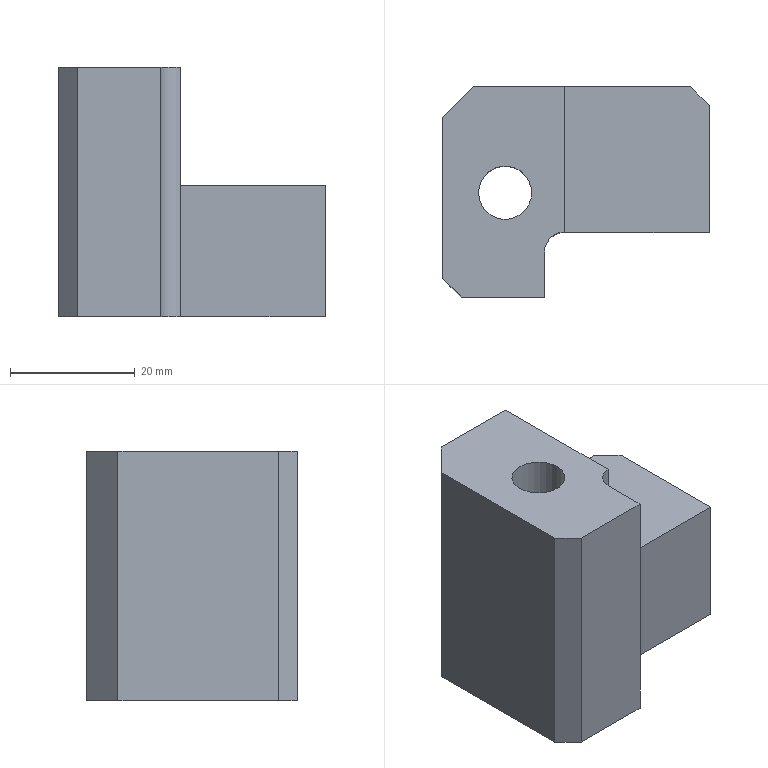Part | NX | features PS-3 2 | 1 solid | 17 faces | box 42.7 x 33.7 x 40 mm | volume 32158 mm3 | plane 14 | cylinder 3 | commonest cylinder face diameters 6.4 x1 8.5 x1 14.5 x1
STEP:
#1=CARTESIAN_POINT('',(2343.858,-896.807,900.716));
#2=VERTEX_POINT('',#1);
#3=CARTESIAN_POINT('',(2348.108,-896.807,900.716));
#4=DIRECTION('',(0.,0.,-1.));
#5=DIRECTION('',(-1.,0.,0.));
#6=AXIS2_PLACEMENT_3D('',#3,#4,#5);
#7=CIRCLE('',#6,4.25);
#8=EDGE_CURVE('',#2,#2,#7,.F.);
#9=ORIENTED_EDGE('',*,*,#8,.T.);
#10=EDGE_LOOP('',(#9));
#11=FACE_BOUND('',#10,.T.);
#12=CARTESIAN_POINT('',(2343.858,-896.807,871.716));
#13=VERTEX_POINT('',#12);
#14=CARTESIAN_POINT('',(2348.108,-896.807,871.716));
#15=DIRECTION('',(0.,0.,1.));
#16=DIRECTION('',(-1.,0.,0.));
#17=AXIS2_PLACEMENT_3D('',#14,#15,#16);
#18=CIRCLE('',#17,4.25);
#19=EDGE_CURVE('',#13,#13,#18,.T.);
#20=ORIENTED_EDGE('',*,*,#19,.F.);
#21=EDGE_LOOP('',(#20));
#22=FACE_BOUND('',#21,.T.);
#23=CARTESIAN_POINT('',(2348.108,-896.807,891.716));
#24=DIRECTION('',(0.,0.,-1.));
#25=DIRECTION('',(-1.,0.,0.));
#26=AXIS2_PLACEMENT_3D('',#23,#24,#25);
#27=CYLINDRICAL_SURFACE('',#26,4.25);
#28=ADVANCED_FACE('',(#11,#22),#27,.F.);
#29=ORIENTED_EDGE('',*,*,#8,.F.);
#30=EDGE_LOOP('',(#29));
#31=FACE_BOUND('',#30,.T.);
#32=CARTESIAN_POINT('',(2357.608,-903.107,900.716));
#33=VERTEX_POINT('',#32);
#34=CARTESIAN_POINT('',(2354.408,-906.307,900.716));
#35=VERTEX_POINT('',#34);
#36=CARTESIAN_POINT('',(2357.608,-906.307,900.716));
#37=DIRECTION('',(0.,0.,-1.));
#38=DIRECTION('',(-1.,0.,0.));
#39=AXIS2_PLACEMENT_3D('',#36,#37,#38);
#40=CIRCLE('',#39,3.2);
#41=EDGE_CURVE('',#33,#35,#40,.F.);
#42=ORIENTED_EDGE('',*,*,#41,.F.);
#43=CARTESIAN_POINT('',(2357.608,-879.807,900.716));
#44=VERTEX_POINT('',#43);
#45=CARTESIAN_POINT('',(2357.608,-891.807,900.716));
#46=DIRECTION('',(0.,-1.,0.));
#47=VECTOR('',#46,1000.);
#48=LINE('',#45,#47);
#49=EDGE_CURVE('',#44,#33,#48,.T.);
#50=ORIENTED_EDGE('',*,*,#49,.F.);
#51=CARTESIAN_POINT('',(2343.108,-879.807,900.716));
#52=VERTEX_POINT('',#51);
#53=CARTESIAN_POINT('',(2375.108,-879.807,900.716));
#54=DIRECTION('',(-1.,0.,0.));
#55=VECTOR('',#54,1000.);
#56=LINE('',#53,#55);
#57=EDGE_CURVE('',#44,#52,#56,.T.);
#58=ORIENTED_EDGE('',*,*,#57,.T.);
#59=CARTESIAN_POINT('',(2338.108,-884.807,900.716));
#60=VERTEX_POINT('',#59);
#61=CARTESIAN_POINT('',(2356.858,-866.057,900.716));
#62=DIRECTION('',(-0.7071,-0.7071,0.));
#63=VECTOR('',#62,1000.);
#64=LINE('',#61,#63);
#65=EDGE_CURVE('',#60,#52,#64,.F.);
#66=ORIENTED_EDGE('',*,*,#65,.F.);
#67=CARTESIAN_POINT('',(2338.108,-910.507,900.716));
#68=VERTEX_POINT('',#67);
#69=CARTESIAN_POINT('',(2338.108,-884.307,900.716));
#70=DIRECTION('',(0.,-1.,0.));
#71=VECTOR('',#70,1000.);
#72=LINE('',#69,#71);
#73=EDGE_CURVE('',#60,#68,#72,.T.);
#74=ORIENTED_EDGE('',*,*,#73,.T.);
#75=CARTESIAN_POINT('',(2341.108,-913.507,900.716));
#76=VERTEX_POINT('',#75);
#77=CARTESIAN_POINT('',(2343.508,-915.907,900.716));
#78=DIRECTION('',(0.7071,-0.7071,0.));
#79=VECTOR('',#78,1000.);
#80=LINE('',#77,#79);
#81=EDGE_CURVE('',#76,#68,#80,.F.);
#82=ORIENTED_EDGE('',*,*,#81,.F.);
#83=CARTESIAN_POINT('',(2354.408,-913.507,900.716));
#84=VERTEX_POINT('',#83);
#85=CARTESIAN_POINT('',(2375.108,-913.507,900.716));
#86=DIRECTION('',(1.,0.,0.));
#87=VECTOR('',#86,1000.);
#88=LINE('',#85,#87);
#89=EDGE_CURVE('',#76,#84,#88,.T.);
#90=ORIENTED_EDGE('',*,*,#89,.T.);
#91=CARTESIAN_POINT('',(2354.408,-912.463,900.716));
#92=DIRECTION('',(0.,1.,0.));
#93=VECTOR('',#92,1000.);
#94=LINE('',#91,#93);
#95=EDGE_CURVE('',#84,#35,#94,.T.);
#96=ORIENTED_EDGE('',*,*,#95,.T.);
#97=EDGE_LOOP('',(#42,#50,#58,#66,#74,#82,#90,#96));
#98=FACE_BOUND('',#97,.T.);
#99=CARTESIAN_POINT('',(2375.108,-884.307,900.716));
#100=DIRECTION('',(0.,0.,-1.));
#101=DIRECTION('',(-1.,0.,0.));
#102=AXIS2_PLACEMENT_3D('',#99,#100,#101);
#103=PLANE('',#102);
#104=ADVANCED_FACE('',(#31,#98),#103,.F.);
#105=CARTESIAN_POINT('',(2343.108,-879.807,860.716));
#106=VERTEX_POINT('',#105);
#107=CARTESIAN_POINT('',(2343.108,-879.807,860.716));
#108=DIRECTION('',(0.,0.,-1.));
#109=VECTOR('',#108,1000.);
#110=LINE('',#107,#109);
#111=EDGE_CURVE('',#52,#106,#110,.T.);
#112=ORIENTED_EDGE('',*,*,#111,.T.);
#113=CARTESIAN_POINT('',(2338.108,-884.807,860.716));
#114=VERTEX_POINT('',#113);
#115=CARTESIAN_POINT('',(2356.858,-866.057,860.716));
#116=DIRECTION('',(0.7071,0.7071,0.));
#117=VECTOR('',#116,1000.);
#118=LINE('',#115,#117);
#119=EDGE_CURVE('',#106,#114,#118,.F.);
#120=ORIENTED_EDGE('',*,*,#119,.T.);
#121=CARTESIAN_POINT('',(2338.108,-884.807,860.716));
#122=DIRECTION('',(0.,0.,1.));
#123=VECTOR('',#122,1000.);
#124=LINE('',#121,#123);
#125=EDGE_CURVE('',#114,#60,#124,.T.);
#126=ORIENTED_EDGE('',*,*,#125,.T.);
#127=ORIENTED_EDGE('',*,*,#65,.T.);
#128=EDGE_LOOP('',(#112,#120,#126,#127));
#129=FACE_BOUND('',#128,.T.);
#130=CARTESIAN_POINT('',(2338.108,-884.807,860.716));
#131=DIRECTION('',(0.7071,-0.7071,0.));
#132=DIRECTION('',(0.,0.,1.));
#133=AXIS2_PLACEMENT_3D('',#130,#131,#132);
#134=PLANE('',#133);
#135=ADVANCED_FACE('',(#129),#134,.F.);
#136=CARTESIAN_POINT('',(2338.108,-910.507,860.716));
#137=VERTEX_POINT('',#136);
#138=CARTESIAN_POINT('',(2338.108,-910.507,860.716));
#139=DIRECTION('',(0.,0.,1.));
#140=VECTOR('',#139,1000.);
#141=LINE('',#138,#140);
#142=EDGE_CURVE('',#68,#137,#141,.F.);
#143=ORIENTED_EDGE('',*,*,#142,.T.);
#144=CARTESIAN_POINT('',(2341.108,-913.507,860.716));
#145=VERTEX_POINT('',#144);
#146=CARTESIAN_POINT('',(2341.108,-913.507,860.716));
#147=DIRECTION('',(-0.7071,0.7071,0.));
#148=VECTOR('',#147,1000.);
#149=LINE('',#146,#148);
#150=EDGE_CURVE('',#137,#145,#149,.F.);
#151=ORIENTED_EDGE('',*,*,#150,.T.);
#152=CARTESIAN_POINT('',(2341.108,-913.507,860.716));
#153=DIRECTION('',(0.,0.,-1.));
#154=VECTOR('',#153,1000.);
#155=LINE('',#152,#154);
#156=EDGE_CURVE('',#145,#76,#155,.F.);
#157=ORIENTED_EDGE('',*,*,#156,.T.);
#158=ORIENTED_EDGE('',*,*,#81,.T.);
#159=EDGE_LOOP('',(#143,#151,#157,#158));
#160=FACE_BOUND('',#159,.T.);
#161=CARTESIAN_POINT('',(2341.108,-913.507,860.716));
#162=DIRECTION('',(0.7071,0.7071,0.));
#163=DIRECTION('',(-0.7071,0.7071,0.));
#164=AXIS2_PLACEMENT_3D('',#161,#162,#163);
#165=PLANE('',#164);
#166=ADVANCED_FACE('',(#160),#165,.F.);
#167=CARTESIAN_POINT('',(2354.408,-906.307,860.716));
#168=VERTEX_POINT('',#167);
#169=CARTESIAN_POINT('',(2354.408,-906.307,935.716));
#170=DIRECTION('',(0.,0.,1.));
#171=VECTOR('',#170,1000.);
#172=LINE('',#169,#171);
#173=EDGE_CURVE('',#168,#35,#172,.T.);
#174=ORIENTED_EDGE('',*,*,#173,.F.);
#175=CARTESIAN_POINT('',(2357.608,-903.107,860.716));
#176=VERTEX_POINT('',#175);
#177=CARTESIAN_POINT('',(2357.608,-906.307,860.716));
#178=DIRECTION('',(0.,0.,1.));
#179=DIRECTION('',(-1.,0.,0.));
#180=AXIS2_PLACEMENT_3D('',#177,#178,#179);
#181=CIRCLE('',#180,3.2);
#182=EDGE_CURVE('',#168,#176,#181,.F.);
#183=ORIENTED_EDGE('',*,*,#182,.T.);
#184=CARTESIAN_POINT('',(2357.608,-903.107,881.716));
#185=VERTEX_POINT('',#184);
#186=CARTESIAN_POINT('',(2357.608,-903.107,935.716));
#187=DIRECTION('',(0.,0.,1.));
#188=VECTOR('',#187,1000.);
#189=LINE('',#186,#188);
#190=EDGE_CURVE('',#185,#176,#189,.F.);
#191=ORIENTED_EDGE('',*,*,#190,.F.);
#192=CARTESIAN_POINT('',(2357.608,-903.107,912.416));
#193=DIRECTION('',(0.,0.,-1.));
#194=VECTOR('',#193,1000.);
#195=LINE('',#192,#194);
#196=EDGE_CURVE('',#33,#185,#195,.T.);
#197=ORIENTED_EDGE('',*,*,#196,.F.);
#198=ORIENTED_EDGE('',*,*,#41,.T.);
#199=EDGE_LOOP('',(#174,#183,#191,#197,#198));
#200=FACE_BOUND('',#199,.T.);
#201=CARTESIAN_POINT('',(2357.608,-906.307,935.716));
#202=DIRECTION('',(0.,0.,1.));
#203=DIRECTION('',(1.,0.,0.));
#204=AXIS2_PLACEMENT_3D('',#201,#202,#203);
#205=CYLINDRICAL_SURFACE('',#204,3.2);
#206=ADVANCED_FACE('',(#200),#205,.F.);
#207=CARTESIAN_POINT('',(2354.408,-913.507,860.716));
#208=VERTEX_POINT('',#207);
#209=CARTESIAN_POINT('',(2354.408,-913.507,935.716));
#210=DIRECTION('',(0.,0.,1.));
#211=VECTOR('',#210,1000.);
#212=LINE('',#209,#211);
#213=EDGE_CURVE('',#208,#84,#212,.T.);
#214=ORIENTED_EDGE('',*,*,#213,.F.);
#215=CARTESIAN_POINT('',(2354.408,-884.307,860.716));
#216=DIRECTION('',(0.,1.,0.));
#217=VECTOR('',#216,1000.);
#218=LINE('',#215,#217);
#219=EDGE_CURVE('',#208,#168,#218,.T.);
#220=ORIENTED_EDGE('',*,*,#219,.T.);
#221=ORIENTED_EDGE('',*,*,#173,.T.);
#222=ORIENTED_EDGE('',*,*,#95,.F.);
#223=EDGE_LOOP('',(#214,#220,#221,#222));
#224=FACE_BOUND('',#223,.T.);
#225=CARTESIAN_POINT('',(2354.408,-912.463,935.716));
#226=DIRECTION('',(1.,0.,0.));
#227=DIRECTION('',(0.,0.,-1.));
#228=AXIS2_PLACEMENT_3D('',#225,#226,#227);
#229=PLANE('',#228);
#230=ADVANCED_FACE('',(#224),#229,.T.);
#231=CARTESIAN_POINT('',(2380.808,-903.107,881.716));
#232=VERTEX_POINT('',#231);
#233=CARTESIAN_POINT('',(2380.108,-903.107,881.716));
#234=DIRECTION('',(-1.,0.,0.));
#235=VECTOR('',#234,1000.);
#236=LINE('',#233,#235);
#237=EDGE_CURVE('',#232,#185,#236,.T.);
#238=ORIENTED_EDGE('',*,*,#237,.T.);
#239=ORIENTED_EDGE('',*,*,#190,.T.);
#240=CARTESIAN_POINT('',(2380.808,-903.107,860.716));
#241=VERTEX_POINT('',#240);
#242=CARTESIAN_POINT('',(2375.108,-903.107,860.716));
#243=DIRECTION('',(1.,0.,0.));
#244=VECTOR('',#243,1000.);
#245=LINE('',#242,#244);
#246=EDGE_CURVE('',#176,#241,#245,.T.);
#247=ORIENTED_EDGE('',*,*,#246,.T.);
#248=CARTESIAN_POINT('',(2380.808,-903.107,860.716));
#249=DIRECTION('',(0.,0.,-1.));
#250=VECTOR('',#249,1000.);
#251=LINE('',#248,#250);
#252=EDGE_CURVE('',#232,#241,#251,.T.);
#253=ORIENTED_EDGE('',*,*,#252,.F.);
#254=EDGE_LOOP('',(#238,#239,#247,#253));
#255=FACE_BOUND('',#254,.T.);
#256=CARTESIAN_POINT('',(2380.108,-903.107,935.716));
#257=DIRECTION('',(0.,1.,0.));
#258=DIRECTION('',(0.,0.,1.));
#259=AXIS2_PLACEMENT_3D('',#256,#257,#258);
#260=PLANE('',#259);
#261=ADVANCED_FACE('',(#255),#260,.F.);
#262=ORIENTED_EDGE('',*,*,#156,.F.);
#263=CARTESIAN_POINT('',(2375.108,-913.507,860.716));
#264=DIRECTION('',(1.,0.,0.));
#265=VECTOR('',#264,1000.);
#266=LINE('',#263,#265);
#267=EDGE_CURVE('',#145,#208,#266,.T.);
#268=ORIENTED_EDGE('',*,*,#267,.T.);
#269=ORIENTED_EDGE('',*,*,#213,.T.);
#270=ORIENTED_EDGE('',*,*,#89,.F.);
#271=EDGE_LOOP('',(#262,#268,#269,#270));
#272=FACE_BOUND('',#271,.T.);
#273=CARTESIAN_POINT('',(2357.608,-913.507,860.716));
#274=DIRECTION('',(0.,1.,0.));
#275=DIRECTION('',(0.,0.,-1.));
#276=AXIS2_PLACEMENT_3D('',#273,#274,#275);
#277=PLANE('',#276);
#278=ADVANCED_FACE('',(#272),#277,.F.);
#279=ORIENTED_EDGE('',*,*,#125,.F.);
#280=CARTESIAN_POINT('',(2338.108,-906.307,860.716));
#281=DIRECTION('',(0.,-1.,0.));
#282=VECTOR('',#281,1000.);
#283=LINE('',#280,#282);
#284=EDGE_CURVE('',#114,#137,#283,.T.);
#285=ORIENTED_EDGE('',*,*,#284,.T.);
#286=ORIENTED_EDGE('',*,*,#142,.F.);
#287=ORIENTED_EDGE('',*,*,#73,.F.);
#288=EDGE_LOOP('',(#279,#285,#286,#287));
#289=FACE_BOUND('',#288,.T.);
#290=CARTESIAN_POINT('',(2338.108,-906.307,860.716));
#291=DIRECTION('',(1.,0.,0.));
#292=DIRECTION('',(0.,0.,-1.));
#293=AXIS2_PLACEMENT_3D('',#290,#291,#292);
#294=PLANE('',#293);
#295=ADVANCED_FACE('',(#289),#294,.F.);
#296=ORIENTED_EDGE('',*,*,#57,.F.);
#297=CARTESIAN_POINT('',(2357.608,-879.807,881.716));
#298=VERTEX_POINT('',#297);
#299=CARTESIAN_POINT('',(2357.608,-879.807,912.416));
#300=DIRECTION('',(0.,0.,1.));
#301=VECTOR('',#300,1000.);
#302=LINE('',#299,#301);
#303=EDGE_CURVE('',#298,#44,#302,.T.);
#304=ORIENTED_EDGE('',*,*,#303,.F.);
#305=CARTESIAN_POINT('',(2377.808,-879.807,881.716));
#306=VERTEX_POINT('',#305);
#307=CARTESIAN_POINT('',(2359.458,-879.807,881.716));
#308=DIRECTION('',(-1.,0.,0.));
#309=VECTOR('',#308,1000.);
#310=LINE('',#307,#309);
#311=EDGE_CURVE('',#306,#298,#310,.T.);
#312=ORIENTED_EDGE('',*,*,#311,.F.);
#313=CARTESIAN_POINT('',(2377.808,-879.807,860.716));
#314=VERTEX_POINT('',#313);
#315=CARTESIAN_POINT('',(2377.808,-879.807,860.716));
#316=DIRECTION('',(0.,0.,-1.));
#317=VECTOR('',#316,1000.);
#318=LINE('',#315,#317);
#319=EDGE_CURVE('',#314,#306,#318,.F.);
#320=ORIENTED_EDGE('',*,*,#319,.F.);
#321=CARTESIAN_POINT('',(2375.108,-879.807,860.716));
#322=DIRECTION('',(-1.,0.,0.));
#323=VECTOR('',#322,1000.);
#324=LINE('',#321,#323);
#325=EDGE_CURVE('',#314,#106,#324,.T.);
#326=ORIENTED_EDGE('',*,*,#325,.T.);
#327=ORIENTED_EDGE('',*,*,#111,.F.);
#328=EDGE_LOOP('',(#296,#304,#312,#320,#326,#327));
#329=FACE_BOUND('',#328,.T.);
#330=CARTESIAN_POINT('',(2375.108,-879.807,860.716));
#331=DIRECTION('',(0.,-1.,0.));
#332=DIRECTION('',(0.,0.,1.));
#333=AXIS2_PLACEMENT_3D('',#330,#331,#332);
#334=PLANE('',#333);
#335=ADVANCED_FACE('',(#329),#334,.F.);
#336=ORIENTED_EDGE('',*,*,#196,.T.);
#337=CARTESIAN_POINT('',(2357.608,-896.657,881.716));
#338=DIRECTION('',(0.,1.,0.));
#339=VECTOR('',#338,1000.);
#340=LINE('',#337,#339);
#341=EDGE_CURVE('',#185,#298,#340,.T.);
#342=ORIENTED_EDGE('',*,*,#341,.T.);
#343=ORIENTED_EDGE('',*,*,#303,.T.);
#344=ORIENTED_EDGE('',*,*,#49,.T.);
#345=EDGE_LOOP('',(#336,#342,#343,#344));
#346=FACE_BOUND('',#345,.T.);
#347=CARTESIAN_POINT('',(2357.608,-891.807,912.416));
#348=DIRECTION('',(-1.,0.,0.));
#349=DIRECTION('',(0.,0.,1.));
#350=AXIS2_PLACEMENT_3D('',#347,#348,#349);
#351=PLANE('',#350);
#352=ADVANCED_FACE('',(#346),#351,.F.);
#353=ORIENTED_EDGE('',*,*,#325,.F.);
#354=CARTESIAN_POINT('',(2380.808,-882.807,860.716));
#355=VERTEX_POINT('',#354);
#356=CARTESIAN_POINT('',(2377.808,-879.807,860.716));
#357=DIRECTION('',(0.7071,-0.7071,0.));
#358=VECTOR('',#357,1000.);
#359=LINE('',#356,#358);
#360=EDGE_CURVE('',#355,#314,#359,.F.);
#361=ORIENTED_EDGE('',*,*,#360,.F.);
#362=CARTESIAN_POINT('',(2380.808,-884.307,860.716));
#363=DIRECTION('',(0.,1.,0.));
#364=VECTOR('',#363,1000.);
#365=LINE('',#362,#364);
#366=EDGE_CURVE('',#241,#355,#365,.T.);
#367=ORIENTED_EDGE('',*,*,#366,.F.);
#368=ORIENTED_EDGE('',*,*,#246,.F.);
#369=ORIENTED_EDGE('',*,*,#182,.F.);
#370=ORIENTED_EDGE('',*,*,#219,.F.);
#371=ORIENTED_EDGE('',*,*,#267,.F.);
#372=ORIENTED_EDGE('',*,*,#150,.F.);
#373=ORIENTED_EDGE('',*,*,#284,.F.);
#374=ORIENTED_EDGE('',*,*,#119,.F.);
#375=EDGE_LOOP('',(#353,#361,#367,#368,#369,#370,#371,#372,#373,#374));
#376=FACE_BOUND('',#375,.T.);
#377=CARTESIAN_POINT('',(2340.858,-896.807,860.716));
#378=VERTEX_POINT('',#377);
#379=CARTESIAN_POINT('',(2348.108,-896.807,860.716));
#380=DIRECTION('',(0.,0.,1.));
#381=DIRECTION('',(-1.,0.,0.));
#382=AXIS2_PLACEMENT_3D('',#379,#380,#381);
#383=CIRCLE('',#382,7.25);
#384=EDGE_CURVE('',#378,#378,#383,.T.);
#385=ORIENTED_EDGE('',*,*,#384,.T.);
#386=EDGE_LOOP('',(#385));
#387=FACE_BOUND('',#386,.T.);
#388=CARTESIAN_POINT('',(2375.108,-884.307,860.716));
#389=DIRECTION('',(0.,0.,-1.));
#390=DIRECTION('',(-1.,0.,0.));
#391=AXIS2_PLACEMENT_3D('',#388,#389,#390);
#392=PLANE('',#391);
#393=ADVANCED_FACE('',(#376,#387),#392,.T.);
#394=ORIENTED_EDGE('',*,*,#384,.F.);
#395=EDGE_LOOP('',(#394));
#396=FACE_BOUND('',#395,.T.);
#397=CARTESIAN_POINT('',(2340.858,-896.807,871.716));
#398=VERTEX_POINT('',#397);
#399=CARTESIAN_POINT('',(2348.108,-896.807,871.716));
#400=DIRECTION('',(0.,0.,1.));
#401=DIRECTION('',(-1.,0.,0.));
#402=AXIS2_PLACEMENT_3D('',#399,#400,#401);
#403=CIRCLE('',#402,7.25);
#404=EDGE_CURVE('',#398,#398,#403,.F.);
#405=ORIENTED_EDGE('',*,*,#404,.F.);
#406=EDGE_LOOP('',(#405));
#407=FACE_BOUND('',#406,.T.);
#408=CARTESIAN_POINT('',(2348.108,-896.807,871.716));
#409=DIRECTION('',(0.,0.,-1.));
#410=DIRECTION('',(-1.,0.,0.));
#411=AXIS2_PLACEMENT_3D('',#408,#409,#410);
#412=CYLINDRICAL_SURFACE('',#411,7.25);
#413=ADVANCED_FACE('',(#396,#407),#412,.F.);
#414=ORIENTED_EDGE('',*,*,#19,.T.);
#415=EDGE_LOOP('',(#414));
#416=FACE_BOUND('',#415,.T.);
#417=ORIENTED_EDGE('',*,*,#404,.T.);
#418=EDGE_LOOP('',(#417));
#419=FACE_BOUND('',#418,.T.);
#420=CARTESIAN_POINT('',(2348.108,-896.807,871.716));
#421=DIRECTION('',(0.,0.,-1.));
#422=DIRECTION('',(-1.,0.,0.));
#423=AXIS2_PLACEMENT_3D('',#420,#421,#422);
#424=PLANE('',#423);
#425=ADVANCED_FACE('',(#416,#419),#424,.T.);
#426=ORIENTED_EDGE('',*,*,#341,.F.);
#427=ORIENTED_EDGE('',*,*,#237,.F.);
#428=CARTESIAN_POINT('',(2380.808,-882.807,881.716));
#429=VERTEX_POINT('',#428);
#430=CARTESIAN_POINT('',(2380.808,-896.657,881.716));
#431=DIRECTION('',(0.,1.,0.));
#432=VECTOR('',#431,1000.);
#433=LINE('',#430,#432);
#434=EDGE_CURVE('',#232,#429,#433,.T.);
#435=ORIENTED_EDGE('',*,*,#434,.T.);
#436=CARTESIAN_POINT('',(2377.058,-879.057,881.716));
#437=DIRECTION('',(-0.7071,0.7071,0.));
#438=VECTOR('',#437,1000.);
#439=LINE('',#436,#438);
#440=EDGE_CURVE('',#306,#429,#439,.F.);
#441=ORIENTED_EDGE('',*,*,#440,.F.);
#442=ORIENTED_EDGE('',*,*,#311,.T.);
#443=EDGE_LOOP('',(#426,#427,#435,#441,#442));
#444=FACE_BOUND('',#443,.T.);
#445=CARTESIAN_POINT('',(2359.458,-896.657,881.716));
#446=DIRECTION('',(0.,0.,-1.));
#447=DIRECTION('',(-1.,0.,0.));
#448=AXIS2_PLACEMENT_3D('',#445,#446,#447);
#449=PLANE('',#448);
#450=ADVANCED_FACE('',(#444),#449,.F.);
#451=ORIENTED_EDGE('',*,*,#440,.T.);
#452=CARTESIAN_POINT('',(2380.808,-882.807,860.716));
#453=DIRECTION('',(0.,0.,1.));
#454=VECTOR('',#453,1000.);
#455=LINE('',#452,#454);
#456=EDGE_CURVE('',#429,#355,#455,.F.);
#457=ORIENTED_EDGE('',*,*,#456,.T.);
#458=ORIENTED_EDGE('',*,*,#360,.T.);
#459=ORIENTED_EDGE('',*,*,#319,.T.);
#460=EDGE_LOOP('',(#451,#457,#458,#459));
#461=FACE_BOUND('',#460,.T.);
#462=CARTESIAN_POINT('',(2377.808,-879.807,860.716));
#463=DIRECTION('',(-0.7071,-0.7071,0.));
#464=DIRECTION('',(0.7071,-0.7071,0.));
#465=AXIS2_PLACEMENT_3D('',#462,#463,#464);
#466=PLANE('',#465);
#467=ADVANCED_FACE('',(#461),#466,.F.);
#468=ORIENTED_EDGE('',*,*,#456,.F.);
#469=ORIENTED_EDGE('',*,*,#434,.F.);
#470=ORIENTED_EDGE('',*,*,#252,.T.);
#471=ORIENTED_EDGE('',*,*,#366,.T.);
#472=EDGE_LOOP('',(#468,#469,#470,#471));
#473=FACE_BOUND('',#472,.T.);
#474=CARTESIAN_POINT('',(2380.808,-910.307,860.716));
#475=DIRECTION('',(-1.,0.,0.));
#476=DIRECTION('',(0.,0.,1.));
#477=AXIS2_PLACEMENT_3D('',#474,#475,#476);
#478=PLANE('',#477);
#479=ADVANCED_FACE('',(#473),#478,.F.);
#480=CLOSED_SHELL('',(#28,#104,#135,#166,#206,#230,#261,#278,#295,#335,#352,#393,#413,#425,#450,#467,#479));
#481=MANIFOLD_SOLID_BREP('',#480);
#482=(LENGTH_UNIT()NAMED_UNIT(*)SI_UNIT(.MILLI.,.METRE.));
#483=UNCERTAINTY_MEASURE_WITH_UNIT(LENGTH_MEASURE(0.00001),#482,'','');
#484=(NAMED_UNIT(*)PLANE_ANGLE_UNIT()SI_UNIT($,.RADIAN.));
#485=(NAMED_UNIT(*)SI_UNIT($,.STERADIAN.)SOLID_ANGLE_UNIT());
#486=(GEOMETRIC_REPRESENTATION_CONTEXT(3)GLOBAL_UNCERTAINTY_ASSIGNED_CONTEXT((#483))GLOBAL_UNIT_ASSIGNED_CONTEXT((#482,#484,#485))REPRESENTATION_CONTEXT('',''));
#487=ADVANCED_BREP_SHAPE_REPRESENTATION('',(#481),#486);